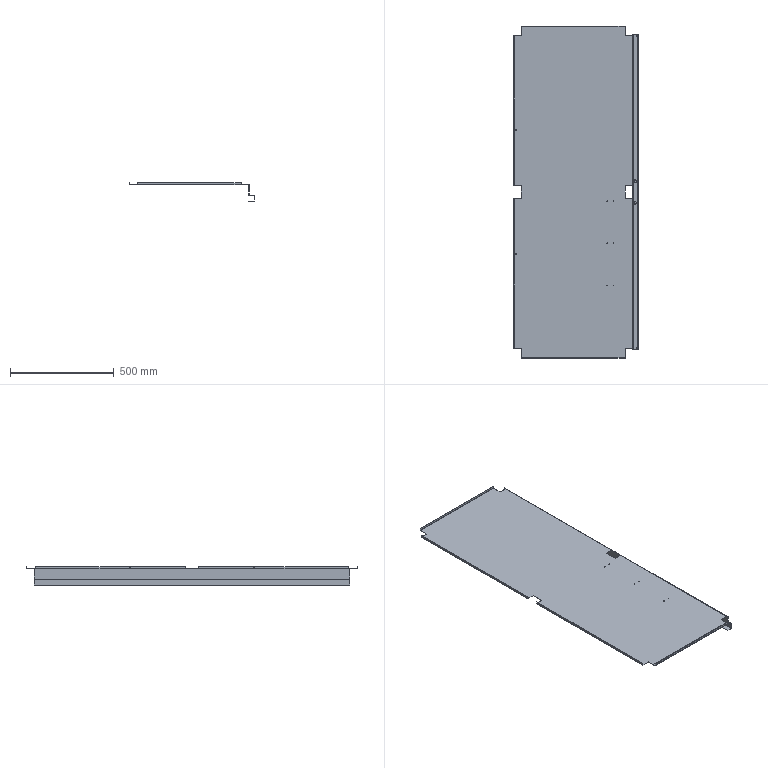Part | STEP file | SOLID | 1 solid | 134 faces | box 599 x 1598 x 90 mm | volume 1123369 mm3 | plane 93 | cylinder 41 | commonest cylinder face diameters 3.3 x12 0.4 x11 2.4 x10 6.1 x4 9 x4